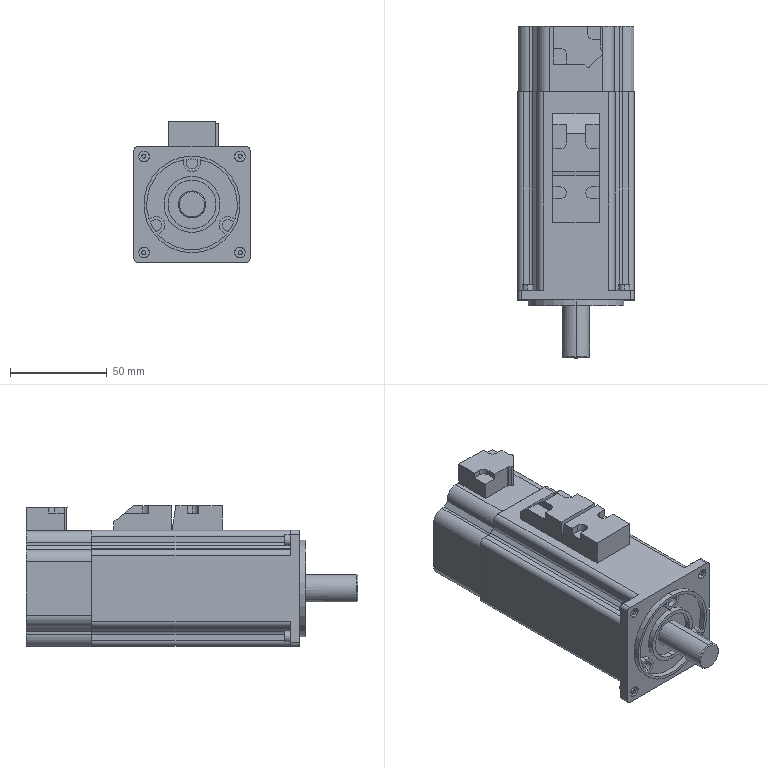Part | SolidWorks | features BaseBody 1 | 1 solid | 234 faces | box 60 x 171.6 x 72.85 mm | volume 479622 mm3 | plane 136 | cylinder 88 | cone 10 | commonest cylinder face diameters 6 x20 5.5 x16 2 x12 4 x12 12 x8 47 x7